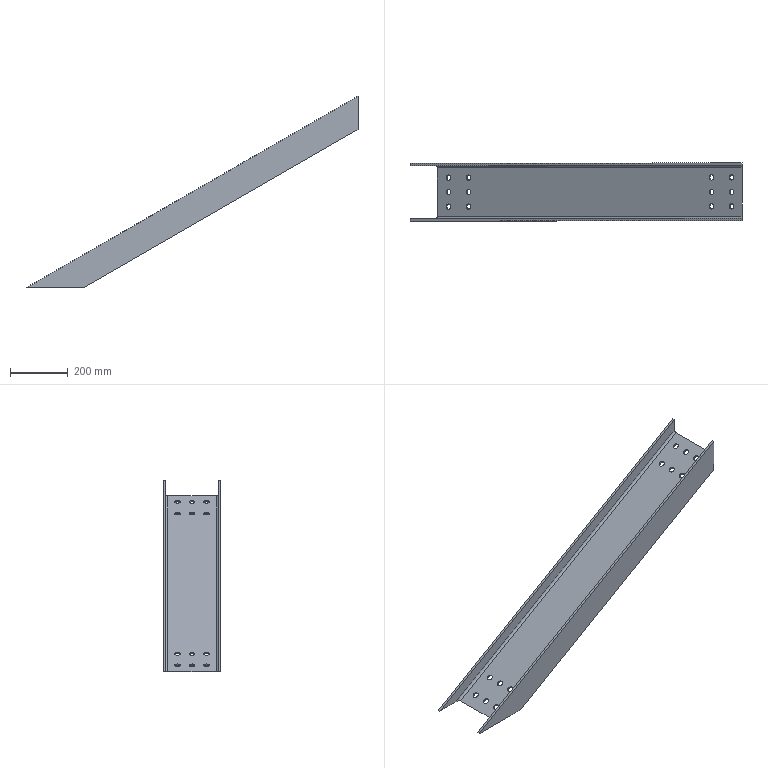Part | STEP file | 粉仓Diagonal Brace梁10_Default<As Machined> | 1 solid | 42 faces | box 1148 x 200 x 662.735 mm | volume 3208282 mm3 | cylinder 28 | plane 14 | commonest cylinder face diameters 19 x24 16 x4